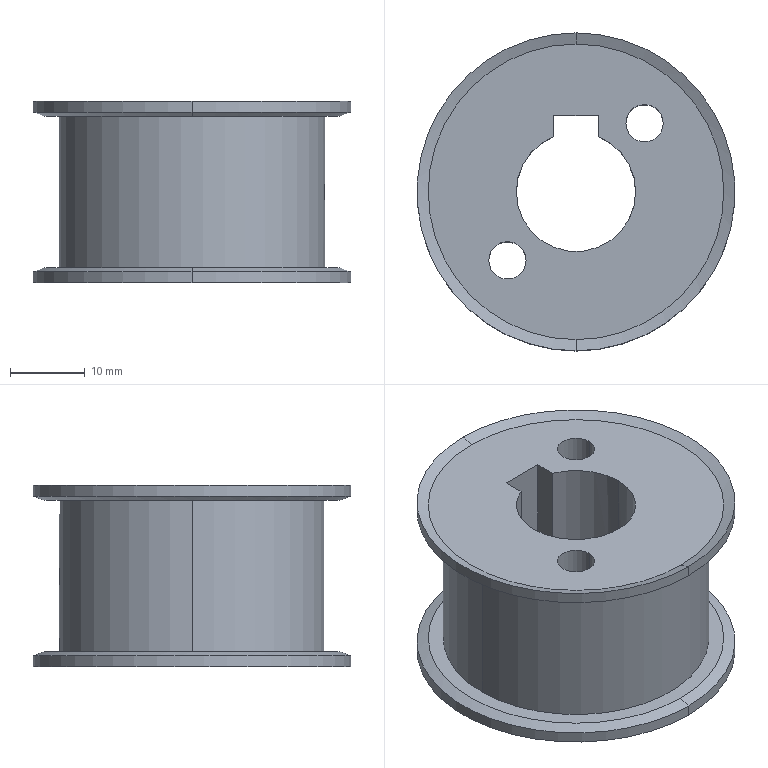Part | STEP file | Driving wheel | 1 solid | 32 faces | box 42.62 x 42.62 x 24.392 mm | volume 18419 mm3 | cylinder 17 | cone 8 | plane 7 | commonest cylinder face diameters 3.3 x4 5 x4 42.62 x4 16 x3 35.62 x2
STEP:
#1=CARTESIAN_POINT('',(-11.692,-9.192,23.3));
#2=VERTEX_POINT('',#1);
#3=CARTESIAN_POINT('',(-6.692,-9.192,23.3));
#4=VERTEX_POINT('',#3);
#5=CARTESIAN_POINT('',(-9.192,-9.192,23.3));
#6=DIRECTION('',(0.,0.,1.));
#7=DIRECTION('',(1.,0.,0.));
#8=AXIS2_PLACEMENT_3D('',#5,#6,#7);
#9=CIRCLE('',#8,2.5);
#10=EDGE_CURVE('',#2,#4,#9,.T.);
#11=ORIENTED_EDGE('',*,*,#10,.T.);
#12=CARTESIAN_POINT('',(-6.692,-9.192,0.));
#13=VERTEX_POINT('',#12);
#14=CARTESIAN_POINT('',(-6.692,-9.192,0.));
#15=DIRECTION('',(0.,0.,-1.));
#16=VECTOR('',#15,1000.);
#17=LINE('',#14,#16);
#18=EDGE_CURVE('',#4,#13,#17,.T.);
#19=ORIENTED_EDGE('',*,*,#18,.T.);
#20=CARTESIAN_POINT('',(-11.692,-9.192,0.));
#21=VERTEX_POINT('',#20);
#22=CARTESIAN_POINT('',(-9.192,-9.192,0.));
#23=DIRECTION('',(0.,0.,-1.));
#24=DIRECTION('',(-1.,0.,0.));
#25=AXIS2_PLACEMENT_3D('',#22,#23,#24);
#26=CIRCLE('',#25,2.5);
#27=EDGE_CURVE('',#13,#21,#26,.T.);
#28=ORIENTED_EDGE('',*,*,#27,.T.);
#29=CARTESIAN_POINT('',(-11.692,-9.192,0.));
#30=DIRECTION('',(0.,0.,-1.));
#31=VECTOR('',#30,1000.);
#32=LINE('',#29,#31);
#33=EDGE_CURVE('',#2,#21,#32,.T.);
#34=ORIENTED_EDGE('',*,*,#33,.F.);
#35=EDGE_LOOP('',(#11,#19,#28,#34));
#36=FACE_OUTER_BOUND('',#35,.T.);
#37=CARTESIAN_POINT('',(-9.192,-9.192,0.));
#38=DIRECTION('',(0.,0.,-1.));
#39=DIRECTION('',(-1.,0.,0.));
#40=AXIS2_PLACEMENT_3D('',#37,#38,#39);
#41=CYLINDRICAL_SURFACE('',#40,2.5);
#42=ADVANCED_FACE('',(#36),#41,.F.);
#43=CARTESIAN_POINT('',(6.692,9.192,23.3));
#44=VERTEX_POINT('',#43);
#45=CARTESIAN_POINT('',(11.692,9.192,23.3));
#46=VERTEX_POINT('',#45);
#47=CARTESIAN_POINT('',(9.192,9.192,23.3));
#48=DIRECTION('',(0.,0.,1.));
#49=DIRECTION('',(1.,0.,0.));
#50=AXIS2_PLACEMENT_3D('',#47,#48,#49);
#51=CIRCLE('',#50,2.5);
#52=EDGE_CURVE('',#44,#46,#51,.T.);
#53=ORIENTED_EDGE('',*,*,#52,.T.);
#54=CARTESIAN_POINT('',(11.692,9.192,0.));
#55=VERTEX_POINT('',#54);
#56=CARTESIAN_POINT('',(11.692,9.192,0.));
#57=DIRECTION('',(0.,0.,-1.));
#58=VECTOR('',#57,1000.);
#59=LINE('',#56,#58);
#60=EDGE_CURVE('',#46,#55,#59,.T.);
#61=ORIENTED_EDGE('',*,*,#60,.T.);
#62=CARTESIAN_POINT('',(6.692,9.192,0.));
#63=VERTEX_POINT('',#62);
#64=CARTESIAN_POINT('',(9.192,9.192,0.));
#65=DIRECTION('',(0.,0.,-1.));
#66=DIRECTION('',(-1.,0.,0.));
#67=AXIS2_PLACEMENT_3D('',#64,#65,#66);
#68=CIRCLE('',#67,2.5);
#69=EDGE_CURVE('',#55,#63,#68,.T.);
#70=ORIENTED_EDGE('',*,*,#69,.T.);
#71=CARTESIAN_POINT('',(6.692,9.192,0.));
#72=DIRECTION('',(0.,0.,-1.));
#73=VECTOR('',#72,1000.);
#74=LINE('',#71,#73);
#75=EDGE_CURVE('',#44,#63,#74,.T.);
#76=ORIENTED_EDGE('',*,*,#75,.F.);
#77=EDGE_LOOP('',(#53,#61,#70,#76));
#78=FACE_OUTER_BOUND('',#77,.T.);
#79=CARTESIAN_POINT('',(9.192,9.192,0.));
#80=DIRECTION('',(0.,0.,-1.));
#81=DIRECTION('',(-1.,0.,0.));
#82=AXIS2_PLACEMENT_3D('',#79,#80,#81);
#83=CYLINDRICAL_SURFACE('',#82,2.5);
#84=ADVANCED_FACE('',(#78),#83,.F.);
#85=CARTESIAN_POINT('',(0.,10.25,13.3));
#86=VERTEX_POINT('',#85);
#87=CARTESIAN_POINT('',(0.,10.25,10.));
#88=VERTEX_POINT('',#87);
#89=CARTESIAN_POINT('',(0.,10.25,11.65));
#90=DIRECTION('',(0.,1.,0.));
#91=DIRECTION('',(0.,0.,1.));
#92=AXIS2_PLACEMENT_3D('',#89,#90,#91);
#93=CIRCLE('',#92,1.65);
#94=EDGE_CURVE('',#86,#88,#93,.T.);
#95=ORIENTED_EDGE('',*,*,#94,.F.);
#96=CARTESIAN_POINT('',(0.,17.81,13.3));
#97=VERTEX_POINT('',#96);
#98=CARTESIAN_POINT('',(0.,17.81,13.3));
#99=DIRECTION('',(0.,1.,0.));
#100=VECTOR('',#99,1000.);
#101=LINE('',#98,#100);
#102=EDGE_CURVE('',#86,#97,#101,.T.);
#103=ORIENTED_EDGE('',*,*,#102,.T.);
#104=CARTESIAN_POINT('',(0.,17.81,10.));
#105=VERTEX_POINT('',#104);
#106=CARTESIAN_POINT('',(0.,17.81,10.));
#107=CARTESIAN_POINT('',(0.1091,17.81,10.));
#108=CARTESIAN_POINT('',(0.2163,17.809,10.011));
#109=CARTESIAN_POINT('',(0.4273,17.805,10.053));
#110=CARTESIAN_POINT('',(0.5321,17.802,10.084));
#111=CARTESIAN_POINT('',(0.7319,17.795,10.167));
#112=CARTESIAN_POINT('',(0.8267,17.791,10.218));
#113=CARTESIAN_POINT('',(1.006,17.782,10.338));
#114=CARTESIAN_POINT('',(1.091,17.777,10.407));
#115=CARTESIAN_POINT('',(1.319,17.762,10.636));
#116=CARTESIAN_POINT('',(1.442,17.752,10.82));
#117=CARTESIAN_POINT('',(1.607,17.738,11.217));
#118=CARTESIAN_POINT('',(1.65,17.733,11.434));
#119=CARTESIAN_POINT('',(1.65,17.733,11.757));
#120=CARTESIAN_POINT('',(1.639,17.734,11.866));
#121=CARTESIAN_POINT('',(1.597,17.738,12.078));
#122=CARTESIAN_POINT('',(1.566,17.741,12.181));
#123=CARTESIAN_POINT('',(1.483,17.748,12.381));
#124=CARTESIAN_POINT('',(1.432,17.752,12.477));
#125=CARTESIAN_POINT('',(1.312,17.762,12.656));
#126=CARTESIAN_POINT('',(1.244,17.767,12.739));
#127=CARTESIAN_POINT('',(1.09,17.777,12.894));
#128=CARTESIAN_POINT('',(1.007,17.782,12.962));
#129=CARTESIAN_POINT('',(0.8279,17.791,13.081));
#130=CARTESIAN_POINT('',(0.7314,17.795,13.133));
#131=CARTESIAN_POINT('',(0.5315,17.802,13.216));
#132=CARTESIAN_POINT('',(0.4287,17.805,13.247));
#133=CARTESIAN_POINT('',(0.2171,17.809,13.289));
#134=CARTESIAN_POINT('',(0.1077,17.81,13.3));
#135=CARTESIAN_POINT('',(0.,17.81,13.3));
#136=B_SPLINE_CURVE_WITH_KNOTS('',3,(#106,#107,#108,#109,#110,#111,#112,#113,#114,#115,#116,#117,#118,#119,#120,#121,#122,#123,#124,#125,#126,#127,#128,#129,#130,#131,#132,#133,#134,#135),.UNSPECIFIED.,.F.,.F.,(4,2,2,2,2,2,2,2,2,2,2,2,2,2,4),(0.,0.0003226,0.0006452,0.0009678,0.00129,0.001936,0.002581,0.002903,0.003226,0.003548,0.003871,0.004194,0.004516,0.004839,0.005161),.UNSPECIFIED.);
#137=EDGE_CURVE('',#105,#97,#136,.T.);
#138=ORIENTED_EDGE('',*,*,#137,.F.);
#139=CARTESIAN_POINT('',(0.,17.81,10.));
#140=DIRECTION('',(0.,1.,0.));
#141=VECTOR('',#140,1000.);
#142=LINE('',#139,#141);
#143=EDGE_CURVE('',#88,#105,#142,.T.);
#144=ORIENTED_EDGE('',*,*,#143,.F.);
#145=EDGE_LOOP('',(#95,#103,#138,#144));
#146=FACE_OUTER_BOUND('',#145,.T.);
#147=CARTESIAN_POINT('',(0.,17.81,11.65));
#148=DIRECTION('',(0.,1.,0.));
#149=DIRECTION('',(0.,0.,-1.));
#150=AXIS2_PLACEMENT_3D('',#147,#148,#149);
#151=CYLINDRICAL_SURFACE('',#150,1.65);
#152=ADVANCED_FACE('',(#146),#151,.F.);
#153=CARTESIAN_POINT('',(8.,0.,13.3));
#154=VERTEX_POINT('',#153);
#155=CARTESIAN_POINT('',(8.,0.,10.));
#156=VERTEX_POINT('',#155);
#157=CARTESIAN_POINT('',(8.,0.,13.3));
#158=CARTESIAN_POINT('',(8.,-0.2156,13.3));
#159=CARTESIAN_POINT('',(7.991,-0.4333,13.257));
#160=CARTESIAN_POINT('',(7.967,-0.7313,13.133));
#161=CARTESIAN_POINT('',(7.958,-0.8276,13.082));
#162=CARTESIAN_POINT('',(7.937,-1.007,12.961));
#163=CARTESIAN_POINT('',(7.926,-1.09,12.893));
#164=CARTESIAN_POINT('',(7.903,-1.242,12.741));
#165=CARTESIAN_POINT('',(7.892,-1.312,12.657));
#166=CARTESIAN_POINT('',(7.871,-1.431,12.478));
#167=CARTESIAN_POINT('',(7.862,-1.482,12.384));
#168=CARTESIAN_POINT('',(7.837,-1.607,12.083));
#169=CARTESIAN_POINT('',(7.828,-1.65,11.869));
#170=CARTESIAN_POINT('',(7.828,-1.65,11.542));
#171=CARTESIAN_POINT('',(7.83,-1.639,11.435));
#172=CARTESIAN_POINT('',(7.839,-1.597,11.223));
#173=CARTESIAN_POINT('',(7.845,-1.566,11.118));
#174=CARTESIAN_POINT('',(7.861,-1.483,10.919));
#175=CARTESIAN_POINT('',(7.871,-1.432,10.824));
#176=CARTESIAN_POINT('',(7.892,-1.312,10.644));
#177=CARTESIAN_POINT('',(7.903,-1.243,10.56));
#178=CARTESIAN_POINT('',(7.937,-1.016,10.332));
#179=CARTESIAN_POINT('',(7.959,-0.8325,10.209));
#180=CARTESIAN_POINT('',(7.983,-0.5348,10.085));
#181=CARTESIAN_POINT('',(7.989,-0.4301,10.053));
#182=CARTESIAN_POINT('',(7.998,-0.2172,10.011));
#183=CARTESIAN_POINT('',(8.,-0.1093,10.));
#184=CARTESIAN_POINT('',(8.,0.,10.));
#185=B_SPLINE_CURVE_WITH_KNOTS('',3,(#157,#158,#159,#160,#161,#162,#163,#164,#165,#166,#167,#168,#169,#170,#171,#172,#173,#174,#175,#176,#177,#178,#179,#180,#181,#182,#183,#184),.UNSPECIFIED.,.F.,.F.,(4,2,2,2,2,2,2,2,2,2,2,2,2,4),(0.005173,0.005819,0.006142,0.006465,0.006789,0.007112,0.007758,0.008081,0.008405,0.008728,0.009051,0.009697,0.01002,0.01034),.UNSPECIFIED.);
#186=EDGE_CURVE('',#154,#156,#185,.T.);
#187=ORIENTED_EDGE('',*,*,#186,.F.);
#188=CARTESIAN_POINT('',(17.81,0.,13.3));
#189=VERTEX_POINT('',#188);
#190=CARTESIAN_POINT('',(17.81,0.,13.3));
#191=DIRECTION('',(1.,0.,0.));
#192=VECTOR('',#191,1000.);
#193=LINE('',#190,#192);
#194=EDGE_CURVE('',#154,#189,#193,.T.);
#195=ORIENTED_EDGE('',*,*,#194,.T.);
#196=CARTESIAN_POINT('',(17.81,0.,10.));
#197=VERTEX_POINT('',#196);
#198=CARTESIAN_POINT('',(17.81,0.,10.));
#199=CARTESIAN_POINT('',(17.81,-0.1091,10.));
#200=CARTESIAN_POINT('',(17.809,-0.2163,10.011));
#201=CARTESIAN_POINT('',(17.805,-0.4273,10.053));
#202=CARTESIAN_POINT('',(17.802,-0.5321,10.084));
#203=CARTESIAN_POINT('',(17.795,-0.7319,10.167));
#204=CARTESIAN_POINT('',(17.791,-0.8267,10.218));
#205=CARTESIAN_POINT('',(17.782,-1.006,10.338));
#206=CARTESIAN_POINT('',(17.777,-1.091,10.407));
#207=CARTESIAN_POINT('',(17.762,-1.319,10.636));
#208=CARTESIAN_POINT('',(17.752,-1.442,10.82));
#209=CARTESIAN_POINT('',(17.738,-1.607,11.217));
#210=CARTESIAN_POINT('',(17.733,-1.65,11.434));
#211=CARTESIAN_POINT('',(17.733,-1.65,11.757));
#212=CARTESIAN_POINT('',(17.734,-1.639,11.866));
#213=CARTESIAN_POINT('',(17.738,-1.597,12.078));
#214=CARTESIAN_POINT('',(17.741,-1.566,12.181));
#215=CARTESIAN_POINT('',(17.748,-1.483,12.381));
#216=CARTESIAN_POINT('',(17.752,-1.432,12.477));
#217=CARTESIAN_POINT('',(17.762,-1.312,12.656));
#218=CARTESIAN_POINT('',(17.767,-1.244,12.739));
#219=CARTESIAN_POINT('',(17.777,-1.09,12.894));
#220=CARTESIAN_POINT('',(17.782,-1.007,12.962));
#221=CARTESIAN_POINT('',(17.791,-0.8279,13.081));
#222=CARTESIAN_POINT('',(17.795,-0.7314,13.133));
#223=CARTESIAN_POINT('',(17.802,-0.5315,13.216));
#224=CARTESIAN_POINT('',(17.805,-0.4287,13.247));
#225=CARTESIAN_POINT('',(17.809,-0.2171,13.289));
#226=CARTESIAN_POINT('',(17.81,-0.1077,13.3));
#227=CARTESIAN_POINT('',(17.81,0.,13.3));
#228=B_SPLINE_CURVE_WITH_KNOTS('',3,(#198,#199,#200,#201,#202,#203,#204,#205,#206,#207,#208,#209,#210,#211,#212,#213,#214,#215,#216,#217,#218,#219,#220,#221,#222,#223,#224,#225,#226,#227),.UNSPECIFIED.,.F.,.F.,(4,2,2,2,2,2,2,2,2,2,2,2,2,2,4),(0.,0.0003226,0.0006452,0.0009678,0.00129,0.001936,0.002581,0.002903,0.003226,0.003548,0.003871,0.004194,0.004516,0.004839,0.005161),.UNSPECIFIED.);
#229=EDGE_CURVE('',#197,#189,#228,.T.);
#230=ORIENTED_EDGE('',*,*,#229,.F.);
#231=CARTESIAN_POINT('',(17.81,0.,10.));
#232=DIRECTION('',(1.,0.,0.));
#233=VECTOR('',#232,1000.);
#234=LINE('',#231,#233);
#235=EDGE_CURVE('',#156,#197,#234,.T.);
#236=ORIENTED_EDGE('',*,*,#235,.F.);
#237=EDGE_LOOP('',(#187,#195,#230,#236));
#238=FACE_OUTER_BOUND('',#237,.T.);
#239=CARTESIAN_POINT('',(17.81,0.,11.65));
#240=DIRECTION('',(1.,0.,0.));
#241=DIRECTION('',(0.,0.,-1.));
#242=AXIS2_PLACEMENT_3D('',#239,#240,#241);
#243=CYLINDRICAL_SURFACE('',#242,1.65);
#244=ADVANCED_FACE('',(#238),#243,.F.);
#245=CARTESIAN_POINT('',(-8.,0.,0.));
#246=VERTEX_POINT('',#245);
#247=CARTESIAN_POINT('',(8.,0.,0.));
#248=VERTEX_POINT('',#247);
#249=CARTESIAN_POINT('',(0.,0.,0.));
#250=DIRECTION('',(0.,0.,1.));
#251=DIRECTION('',(1.,0.,0.));
#252=AXIS2_PLACEMENT_3D('',#249,#250,#251);
#253=CIRCLE('',#252,8.);
#254=EDGE_CURVE('',#246,#248,#253,.T.);
#255=ORIENTED_EDGE('',*,*,#254,.F.);
#256=CARTESIAN_POINT('',(-8.,0.,23.3));
#257=VERTEX_POINT('',#256);
#258=CARTESIAN_POINT('',(-8.,0.,-0.546));
#259=DIRECTION('',(0.,0.,1.));
#260=VECTOR('',#259,1000.);
#261=LINE('',#258,#260);
#262=EDGE_CURVE('',#246,#257,#261,.T.);
#263=ORIENTED_EDGE('',*,*,#262,.T.);
#264=CARTESIAN_POINT('',(8.,0.,23.3));
#265=VERTEX_POINT('',#264);
#266=CARTESIAN_POINT('',(0.,0.,23.3));
#267=DIRECTION('',(0.,0.,1.));
#268=DIRECTION('',(1.,0.,0.));
#269=AXIS2_PLACEMENT_3D('',#266,#267,#268);
#270=CIRCLE('',#269,8.);
#271=EDGE_CURVE('',#257,#265,#270,.T.);
#272=ORIENTED_EDGE('',*,*,#271,.T.);
#273=CARTESIAN_POINT('',(8.,0.,-0.546));
#274=DIRECTION('',(0.,0.,1.));
#275=VECTOR('',#274,1000.);
#276=LINE('',#273,#275);
#277=EDGE_CURVE('',#154,#265,#276,.T.);
#278=ORIENTED_EDGE('',*,*,#277,.F.);
#279=ORIENTED_EDGE('',*,*,#186,.T.);
#280=CARTESIAN_POINT('',(8.,0.,-0.546));
#281=DIRECTION('',(0.,0.,1.));
#282=VECTOR('',#281,1000.);
#283=LINE('',#280,#282);
#284=EDGE_CURVE('',#248,#156,#283,.T.);
#285=ORIENTED_EDGE('',*,*,#284,.F.);
#286=EDGE_LOOP('',(#255,#263,#272,#278,#279,#285));
#287=FACE_OUTER_BOUND('',#286,.T.);
#288=CARTESIAN_POINT('',(0.,0.,-0.546));
#289=DIRECTION('',(0.,0.,1.));
#290=DIRECTION('',(1.,0.,0.));
#291=AXIS2_PLACEMENT_3D('',#288,#289,#290);
#292=CYLINDRICAL_SURFACE('',#291,8.);
#293=ADVANCED_FACE('',(#287),#292,.F.);
#294=CARTESIAN_POINT('',(3.,7.416,0.));
#295=VERTEX_POINT('',#294);
#296=CARTESIAN_POINT('',(0.,0.,0.));
#297=DIRECTION('',(0.,0.,1.));
#298=DIRECTION('',(1.,0.,0.));
#299=AXIS2_PLACEMENT_3D('',#296,#297,#298);
#300=CIRCLE('',#299,8.);
#301=EDGE_CURVE('',#248,#295,#300,.T.);
#302=ORIENTED_EDGE('',*,*,#301,.F.);
#303=ORIENTED_EDGE('',*,*,#284,.T.);
#304=CARTESIAN_POINT('',(8.,0.,10.));
#305=CARTESIAN_POINT('',(8.,0.1093,10.));
#306=CARTESIAN_POINT('',(7.998,0.2168,10.011));
#307=CARTESIAN_POINT('',(7.989,0.4281,10.053));
#308=CARTESIAN_POINT('',(7.983,0.5331,10.085));
#309=CARTESIAN_POINT('',(7.967,0.7328,10.168));
#310=CARTESIAN_POINT('',(7.958,0.8274,10.218));
#311=CARTESIAN_POINT('',(7.937,1.007,10.338));
#312=CARTESIAN_POINT('',(7.926,1.091,10.408));
#313=CARTESIAN_POINT('',(7.892,1.319,10.635));
#314=CARTESIAN_POINT('',(7.869,1.442,10.819));
#315=CARTESIAN_POINT('',(7.838,1.606,11.216));
#316=CARTESIAN_POINT('',(7.828,1.65,11.433));
#317=CARTESIAN_POINT('',(7.828,1.65,11.757));
#318=CARTESIAN_POINT('',(7.83,1.639,11.867));
#319=CARTESIAN_POINT('',(7.839,1.597,12.079));
#320=CARTESIAN_POINT('',(7.845,1.566,12.182));
#321=CARTESIAN_POINT('',(7.87,1.441,12.482));
#322=CARTESIAN_POINT('',(7.892,1.32,12.664));
#323=CARTESIAN_POINT('',(7.926,1.09,12.893));
#324=CARTESIAN_POINT('',(7.937,1.007,12.962));
#325=CARTESIAN_POINT('',(7.957,0.8285,13.081));
#326=CARTESIAN_POINT('',(7.967,0.7318,13.133));
#327=CARTESIAN_POINT('',(7.983,0.5324,13.215));
#328=CARTESIAN_POINT('',(7.989,0.4295,13.247));
#329=CARTESIAN_POINT('',(7.998,0.2174,13.289));
#330=CARTESIAN_POINT('',(8.,0.1078,13.3));
#331=CARTESIAN_POINT('',(8.,0.,13.3));
#332=B_SPLINE_CURVE_WITH_KNOTS('',3,(#304,#305,#306,#307,#308,#309,#310,#311,#312,#313,#314,#315,#316,#317,#318,#319,#320,#321,#322,#323,#324,#325,#326,#327,#328,#329,#330,#331),.UNSPECIFIED.,.F.,.F.,(4,2,2,2,2,2,2,2,2,2,2,2,2,4),(0.,0.0003233,0.0006466,0.0009699,0.001293,0.00194,0.002586,0.00291,0.003233,0.003879,0.004203,0.004526,0.004849,0.005173),.UNSPECIFIED.);
#333=EDGE_CURVE('',#156,#154,#332,.T.);
#334=ORIENTED_EDGE('',*,*,#333,.T.);
#335=ORIENTED_EDGE('',*,*,#277,.T.);
#336=CARTESIAN_POINT('',(3.,7.416,23.3));
#337=VERTEX_POINT('',#336);
#338=CARTESIAN_POINT('',(0.,0.,23.3));
#339=DIRECTION('',(0.,0.,1.));
#340=DIRECTION('',(1.,0.,0.));
#341=AXIS2_PLACEMENT_3D('',#338,#339,#340);
#342=CIRCLE('',#341,8.);
#343=EDGE_CURVE('',#265,#337,#342,.T.);
#344=ORIENTED_EDGE('',*,*,#343,.T.);
#345=CARTESIAN_POINT('',(3.,7.416,-0.546));
#346=DIRECTION('',(0.,0.,-1.));
#347=VECTOR('',#346,1000.);
#348=LINE('',#345,#347);
#349=EDGE_CURVE('',#337,#295,#348,.T.);
#350=ORIENTED_EDGE('',*,*,#349,.T.);
#351=EDGE_LOOP('',(#302,#303,#334,#335,#344,#350));
#352=FACE_OUTER_BOUND('',#351,.T.);
#353=CARTESIAN_POINT('',(0.,0.,-0.546));
#354=DIRECTION('',(0.,0.,1.));
#355=DIRECTION('',(1.,0.,0.));
#356=AXIS2_PLACEMENT_3D('',#353,#354,#355);
#357=CYLINDRICAL_SURFACE('',#356,8.);
#358=ADVANCED_FACE('',(#352),#357,.F.);
#359=CARTESIAN_POINT('',(0.,-19.81,1.5));
#360=VERTEX_POINT('',#359);
#361=CARTESIAN_POINT('',(0.,19.81,1.5));
#362=VERTEX_POINT('',#361);
#363=CARTESIAN_POINT('',(0.,0.,1.5));
#364=DIRECTION('',(0.,0.,1.));
#365=DIRECTION('',(0.,-1.,0.));
#366=AXIS2_PLACEMENT_3D('',#363,#364,#365);
#367=CIRCLE('',#366,19.81);
#368=EDGE_CURVE('',#360,#362,#367,.T.);
#369=ORIENTED_EDGE('',*,*,#368,.F.);
#370=CARTESIAN_POINT('',(0.,-21.31,0.954));
#371=VERTEX_POINT('',#370);
#372=CARTESIAN_POINT('',(0.,-21.31,0.954));
#373=DIRECTION('',(0.,-0.9397,-0.342));
#374=VECTOR('',#373,1000.);
#375=LINE('',#372,#374);
#376=EDGE_CURVE('',#360,#371,#375,.T.);
#377=ORIENTED_EDGE('',*,*,#376,.T.);
#378=CARTESIAN_POINT('',(0.,21.31,0.954));
#379=VERTEX_POINT('',#378);
#380=CARTESIAN_POINT('',(0.,0.,0.954));
#381=DIRECTION('',(0.,0.,1.));
#382=DIRECTION('',(0.,-1.,0.));
#383=AXIS2_PLACEMENT_3D('',#380,#381,#382);
#384=CIRCLE('',#383,21.31);
#385=EDGE_CURVE('',#371,#379,#384,.T.);
#386=ORIENTED_EDGE('',*,*,#385,.T.);
#387=CARTESIAN_POINT('',(0.,21.31,0.954));
#388=DIRECTION('',(0.,0.9397,-0.342));
#389=VECTOR('',#388,1000.);
#390=LINE('',#387,#389);
#391=EDGE_CURVE('',#362,#379,#390,.T.);
#392=ORIENTED_EDGE('',*,*,#391,.F.);
#393=EDGE_LOOP('',(#369,#377,#386,#392));
#394=FACE_OUTER_BOUND('',#393,.T.);
#395=CARTESIAN_POINT('',(0.,0.,0.954));
#396=DIRECTION('',(0.,0.,-1.));
#397=DIRECTION('',(0.,1.,0.));
#398=AXIS2_PLACEMENT_3D('',#395,#396,#397);
#399=CONICAL_SURFACE('',#398,21.31,1.222);
#400=ADVANCED_FACE('',(#394),#399,.T.);
#401=CARTESIAN_POINT('',(0.,-21.31,-0.546));
#402=VERTEX_POINT('',#401);
#403=CARTESIAN_POINT('',(0.,21.31,-0.546));
#404=VERTEX_POINT('',#403);
#405=CARTESIAN_POINT('',(0.,0.,-0.546));
#406=DIRECTION('',(0.,0.,1.));
#407=DIRECTION('',(0.,-1.,0.));
#408=AXIS2_PLACEMENT_3D('',#405,#406,#407);
#409=CIRCLE('',#408,21.31);
#410=EDGE_CURVE('',#402,#404,#409,.T.);
#411=ORIENTED_EDGE('',*,*,#410,.T.);
#412=CARTESIAN_POINT('',(0.,21.31,23.3));
#413=DIRECTION('',(0.,0.,1.));
#414=VECTOR('',#413,1000.);
#415=LINE('',#412,#414);
#416=EDGE_CURVE('',#404,#379,#415,.T.);
#417=ORIENTED_EDGE('',*,*,#416,.T.);
#418=ORIENTED_EDGE('',*,*,#385,.F.);
#419=CARTESIAN_POINT('',(0.,-21.31,23.3));
#420=DIRECTION('',(0.,0.,1.));
#421=VECTOR('',#420,1000.);
#422=LINE('',#419,#421);
#423=EDGE_CURVE('',#402,#371,#422,.T.);
#424=ORIENTED_EDGE('',*,*,#423,.F.);
#425=EDGE_LOOP('',(#411,#417,#418,#424));
#426=FACE_OUTER_BOUND('',#425,.T.);
#427=CARTESIAN_POINT('',(0.,0.,23.3));
#428=DIRECTION('',(0.,0.,1.));
#429=DIRECTION('',(0.,-1.,0.));
#430=AXIS2_PLACEMENT_3D('',#427,#428,#429);
#431=CYLINDRICAL_SURFACE('',#430,21.31);
#432=ADVANCED_FACE('',(#426),#431,.T.);
#433=CARTESIAN_POINT('',(0.,19.81,0.));
#434=VERTEX_POINT('',#433);
#435=CARTESIAN_POINT('',(0.,-19.81,0.));
#436=VERTEX_POINT('',#435);
#437=CARTESIAN_POINT('',(0.,0.,0.));
#438=DIRECTION('',(0.,0.,1.));
#439=DIRECTION('',(0.,-1.,0.));
#440=AXIS2_PLACEMENT_3D('',#437,#438,#439);
#441=CIRCLE('',#440,19.81);
#442=EDGE_CURVE('',#434,#436,#441,.T.);
#443=ORIENTED_EDGE('',*,*,#442,.T.);
#444=CARTESIAN_POINT('',(0.,-19.81,0.));
#445=DIRECTION('',(0.,-0.9397,-0.342));
#446=VECTOR('',#445,1000.);
#447=LINE('',#444,#446);
#448=EDGE_CURVE('',#436,#402,#447,.T.);
#449=ORIENTED_EDGE('',*,*,#448,.T.);
#450=CARTESIAN_POINT('',(0.,0.,-0.546));
#451=DIRECTION('',(0.,0.,1.));
#452=DIRECTION('',(0.,-1.,0.));
#453=AXIS2_PLACEMENT_3D('',#450,#451,#452);
#454=CIRCLE('',#453,21.31);
#455=EDGE_CURVE('',#404,#402,#454,.T.);
#456=ORIENTED_EDGE('',*,*,#455,.F.);
#457=CARTESIAN_POINT('',(0.,19.81,0.));
#458=DIRECTION('',(0.,0.9397,-0.342));
#459=VECTOR('',#458,1000.);
#460=LINE('',#457,#459);
#461=EDGE_CURVE('',#434,#404,#460,.T.);
#462=ORIENTED_EDGE('',*,*,#461,.F.);
#463=EDGE_LOOP('',(#443,#449,#456,#462));
#464=FACE_OUTER_BOUND('',#463,.T.);
#465=CARTESIAN_POINT('',(0.,0.,0.));
#466=DIRECTION('',(0.,0.,-1.));
#467=DIRECTION('',(0.,1.,0.));
#468=AXIS2_PLACEMENT_3D('',#465,#466,#467);
#469=CONICAL_SURFACE('',#468,19.81,1.222);
#470=ADVANCED_FACE('',(#464),#469,.F.);
#471=CARTESIAN_POINT('',(0.,19.81,23.3));
#472=VERTEX_POINT('',#471);
#473=CARTESIAN_POINT('',(0.,-19.81,23.3));
#474=VERTEX_POINT('',#473);
#475=CARTESIAN_POINT('',(0.,0.,23.3));
#476=DIRECTION('',(0.,0.,1.));
#477=DIRECTION('',(0.,-1.,0.));
#478=AXIS2_PLACEMENT_3D('',#475,#476,#477);
#479=CIRCLE('',#478,19.81);
#480=EDGE_CURVE('',#472,#474,#479,.T.);
#481=ORIENTED_EDGE('',*,*,#480,.F.);
#482=CARTESIAN_POINT('',(0.,21.31,23.846));
#483=VERTEX_POINT('',#482);
#484=CARTESIAN_POINT('',(0.,21.31,23.846));
#485=DIRECTION('',(0.,0.9397,0.342));
#486=VECTOR('',#485,1000.);
#487=LINE('',#484,#486);
#488=EDGE_CURVE('',#472,#483,#487,.T.);
#489=ORIENTED_EDGE('',*,*,#488,.T.);
#490=CARTESIAN_POINT('',(0.,-21.31,23.846));
#491=VERTEX_POINT('',#490);
#492=CARTESIAN_POINT('',(0.,0.,23.846));
#493=DIRECTION('',(0.,0.,1.));
#494=DIRECTION('',(0.,-1.,0.));
#495=AXIS2_PLACEMENT_3D('',#492,#493,#494);
#496=CIRCLE('',#495,21.31);
#497=EDGE_CURVE('',#483,#491,#496,.T.);
#498=ORIENTED_EDGE('',*,*,#497,.T.);
#499=CARTESIAN_POINT('',(0.,-21.31,23.846));
#500=DIRECTION('',(0.,-0.9397,0.342));
#501=VECTOR('',#500,1000.);
#502=LINE('',#499,#501);
#503=EDGE_CURVE('',#474,#491,#502,.T.);
#504=ORIENTED_EDGE('',*,*,#503,.F.);
#505=EDGE_LOOP('',(#481,#489,#498,#504));
#506=FACE_OUTER_BOUND('',#505,.T.);
#507=CARTESIAN_POINT('',(0.,0.,23.846));
#508=DIRECTION('',(0.,0.,1.));
#509=DIRECTION('',(0.,-1.,0.));
#510=AXIS2_PLACEMENT_3D('',#507,#508,#509);
#511=CONICAL_SURFACE('',#510,21.31,1.222);
#512=ADVANCED_FACE('',(#506),#511,.F.);
#513=CARTESIAN_POINT('',(0.,-21.31,22.346));
#514=VERTEX_POINT('',#513);
#515=CARTESIAN_POINT('',(0.,21.31,22.346));
#516=VERTEX_POINT('',#515);
#517=CARTESIAN_POINT('',(0.,0.,22.346));
#518=DIRECTION('',(0.,0.,1.));
#519=DIRECTION('',(0.,-1.,0.));
#520=AXIS2_PLACEMENT_3D('',#517,#518,#519);
#521=CIRCLE('',#520,21.31);
#522=EDGE_CURVE('',#514,#516,#521,.T.);
#523=ORIENTED_EDGE('',*,*,#522,.T.);
#524=CARTESIAN_POINT('',(0.,21.31,23.3));
#525=DIRECTION('',(0.,0.,1.));
#526=VECTOR('',#525,1000.);
#527=LINE('',#524,#526);
#528=EDGE_CURVE('',#516,#483,#527,.T.);
#529=ORIENTED_EDGE('',*,*,#528,.T.);
#530=CARTESIAN_POINT('',(0.,0.,23.846));
#531=DIRECTION('',(0.,0.,1.));
#532=DIRECTION('',(0.,-1.,0.));
#533=AXIS2_PLACEMENT_3D('',#530,#531,#532);
#534=CIRCLE('',#533,21.31);
#535=EDGE_CURVE('',#491,#483,#534,.T.);
#536=ORIENTED_EDGE('',*,*,#535,.F.);
#537=CARTESIAN_POINT('',(0.,-21.31,23.3));
#538=DIRECTION('',(0.,0.,1.));
#539=VECTOR('',#538,1000.);
#540=LINE('',#537,#539);
#541=EDGE_CURVE('',#514,#491,#540,.T.);
#542=ORIENTED_EDGE('',*,*,#541,.F.);
#543=EDGE_LOOP('',(#523,#529,#536,#542));
#544=FACE_OUTER_BOUND('',#543,.T.);
#545=CARTESIAN_POINT('',(0.,0.,23.3));
#546=DIRECTION('',(0.,0.,1.));
#547=DIRECTION('',(0.,-1.,0.));
#548=AXIS2_PLACEMENT_3D('',#545,#546,#547);
#549=CYLINDRICAL_SURFACE('',#548,21.31);
#550=ADVANCED_FACE('',(#544),#549,.T.);
#551=CARTESIAN_POINT('',(0.,-19.81,21.8));
#552=VERTEX_POINT('',#551);
#553=CARTESIAN_POINT('',(0.,19.81,21.8));
#554=VERTEX_POINT('',#553);
#555=CARTESIAN_POINT('',(0.,0.,21.8));
#556=DIRECTION('',(0.,0.,1.));
#557=DIRECTION('',(0.,-1.,0.));
#558=AXIS2_PLACEMENT_3D('',#555,#556,#557);
#559=CIRCLE('',#558,19.81);
#560=EDGE_CURVE('',#552,#554,#559,.T.);
#561=ORIENTED_EDGE('',*,*,#560,.T.);
#562=CARTESIAN_POINT('',(0.,19.81,21.8));
#563=DIRECTION('',(0.,0.9397,0.342));
#564=VECTOR('',#563,1000.);
#565=LINE('',#562,#564);
#566=EDGE_CURVE('',#554,#516,#565,.T.);
#567=ORIENTED_EDGE('',*,*,#566,.T.);
#568=ORIENTED_EDGE('',*,*,#522,.F.);
#569=CARTESIAN_POINT('',(0.,-19.81,21.8));
#570=DIRECTION('',(0.,-0.9397,0.342));
#571=VECTOR('',#570,1000.);
#572=LINE('',#569,#571);
#573=EDGE_CURVE('',#552,#514,#572,.T.);
#574=ORIENTED_EDGE('',*,*,#573,.F.);
#575=EDGE_LOOP('',(#561,#567,#568,#574));
#576=FACE_OUTER_BOUND('',#575,.T.);
#577=CARTESIAN_POINT('',(0.,0.,21.8));
#578=DIRECTION('',(0.,0.,1.));
#579=DIRECTION('',(0.,-1.,0.));
#580=AXIS2_PLACEMENT_3D('',#577,#578,#579);
#581=CONICAL_SURFACE('',#580,19.81,1.222);
#582=ADVANCED_FACE('',(#576),#581,.T.);
#583=ORIENTED_EDGE('',*,*,#137,.T.);
#584=CARTESIAN_POINT('',(0.,17.81,13.3));
#585=CARTESIAN_POINT('',(-0.2154,17.81,13.3));
#586=CARTESIAN_POINT('',(-0.4325,17.806,13.257));
#587=CARTESIAN_POINT('',(-0.8297,17.792,13.092));
#588=CARTESIAN_POINT('',(-1.014,17.782,12.97));
#589=CARTESIAN_POINT('',(-1.242,17.767,12.742));
#590=CARTESIAN_POINT('',(-1.312,17.762,12.657));
#591=CARTESIAN_POINT('',(-1.432,17.752,12.477));
#592=CARTESIAN_POINT('',(-1.482,17.748,12.383));
#593=CARTESIAN_POINT('',(-1.565,17.741,12.183));
#594=CARTESIAN_POINT('',(-1.597,17.738,12.078));
#595=CARTESIAN_POINT('',(-1.639,17.734,11.867));
#596=CARTESIAN_POINT('',(-1.65,17.733,11.76));
#597=CARTESIAN_POINT('',(-1.65,17.733,11.542));
#598=CARTESIAN_POINT('',(-1.639,17.734,11.435));
#599=CARTESIAN_POINT('',(-1.598,17.738,11.224));
#600=CARTESIAN_POINT('',(-1.566,17.741,11.119));
#601=CARTESIAN_POINT('',(-1.483,17.748,10.919));
#602=CARTESIAN_POINT('',(-1.433,17.752,10.824));
#603=CARTESIAN_POINT('',(-1.313,17.762,10.645));
#604=CARTESIAN_POINT('',(-1.244,17.767,10.56));
#605=CARTESIAN_POINT('',(-1.015,17.782,10.332));
#606=CARTESIAN_POINT('',(-0.8317,17.792,10.209));
#607=CARTESIAN_POINT('',(-0.4348,17.806,10.044));
#608=CARTESIAN_POINT('',(-0.2181,17.81,10.));
#609=CARTESIAN_POINT('',(0.,17.81,10.));
#610=B_SPLINE_CURVE_WITH_KNOTS('',3,(#584,#585,#586,#587,#588,#589,#590,#591,#592,#593,#594,#595,#596,#597,#598,#599,#600,#601,#602,#603,#604,#605,#606,#607,#608,#609),.UNSPECIFIED.,.F.,.F.,(4,2,2,2,2,2,2,2,2,2,2,2,4),(0.005161,0.005806,0.006451,0.006774,0.007096,0.007419,0.007742,0.008064,0.008387,0.008709,0.009032,0.009677,0.01032),.UNSPECIFIED.);
#611=EDGE_CURVE('',#97,#105,#610,.T.);
#612=ORIENTED_EDGE('',*,*,#611,.T.);
#613=EDGE_LOOP('',(#583,#612));
#614=FACE_BOUND('',#613,.T.);
#615=CARTESIAN_POINT('',(17.81,0.,21.8));
#616=VERTEX_POINT('',#615);
#617=CARTESIAN_POINT('',(-17.81,0.,21.8));
#618=VERTEX_POINT('',#617);
#619=CARTESIAN_POINT('',(0.,0.,21.8));
#620=DIRECTION('',(0.,0.,1.));
#621=DIRECTION('',(0.,-1.,0.));
#622=AXIS2_PLACEMENT_3D('',#619,#620,#621);
#623=CIRCLE('',#622,17.81);
#624=EDGE_CURVE('',#616,#618,#623,.T.);
#625=ORIENTED_EDGE('',*,*,#624,.F.);
#626=CARTESIAN_POINT('',(17.81,0.,23.3));
#627=DIRECTION('',(0.,0.,-1.));
#628=VECTOR('',#627,1000.);
#629=LINE('',#626,#628);
#630=EDGE_CURVE('',#616,#189,#629,.T.);
#631=ORIENTED_EDGE('',*,*,#630,.T.);
#632=CARTESIAN_POINT('',(17.81,0.,13.3));
#633=CARTESIAN_POINT('',(17.81,0.2154,13.3));
#634=CARTESIAN_POINT('',(17.806,0.4325,13.257));
#635=CARTESIAN_POINT('',(17.792,0.8297,13.092));
#636=CARTESIAN_POINT('',(17.782,1.014,12.97));
#637=CARTESIAN_POINT('',(17.767,1.242,12.742));
#638=CARTESIAN_POINT('',(17.762,1.312,12.657));
#639=CARTESIAN_POINT('',(17.752,1.432,12.477));
#640=CARTESIAN_POINT('',(17.748,1.482,12.383));
#641=CARTESIAN_POINT('',(17.741,1.565,12.183));
#642=CARTESIAN_POINT('',(17.738,1.597,12.078));
#643=CARTESIAN_POINT('',(17.734,1.639,11.867));
#644=CARTESIAN_POINT('',(17.733,1.65,11.76));
#645=CARTESIAN_POINT('',(17.733,1.65,11.542));
#646=CARTESIAN_POINT('',(17.734,1.639,11.435));
#647=CARTESIAN_POINT('',(17.738,1.598,11.224));
#648=CARTESIAN_POINT('',(17.741,1.566,11.119));
#649=CARTESIAN_POINT('',(17.748,1.483,10.919));
#650=CARTESIAN_POINT('',(17.752,1.433,10.824));
#651=CARTESIAN_POINT('',(17.762,1.313,10.645));
#652=CARTESIAN_POINT('',(17.767,1.244,10.56));
#653=CARTESIAN_POINT('',(17.782,1.015,10.332));
#654=CARTESIAN_POINT('',(17.792,0.8317,10.209));
#655=CARTESIAN_POINT('',(17.806,0.4348,10.044));
#656=CARTESIAN_POINT('',(17.81,0.2181,10.));
#657=CARTESIAN_POINT('',(17.81,0.,10.));
#658=B_SPLINE_CURVE_WITH_KNOTS('',3,(#632,#633,#634,#635,#636,#637,#638,#639,#640,#641,#642,#643,#644,#645,#646,#647,#648,#649,#650,#651,#652,#653,#654,#655,#656,#657),.UNSPECIFIED.,.F.,.F.,(4,2,2,2,2,2,2,2,2,2,2,2,4),(0.005161,0.005806,0.006451,0.006774,0.007096,0.007419,0.007742,0.008064,0.008387,0.008709,0.009032,0.009677,0.01032),.UNSPECIFIED.);
#659=EDGE_CURVE('',#189,#197,#658,.T.);
#660=ORIENTED_EDGE('',*,*,#659,.T.);
#661=CARTESIAN_POINT('',(17.81,0.,1.5));
#662=VERTEX_POINT('',#661);
#663=CARTESIAN_POINT('',(17.81,0.,23.3));
#664=DIRECTION('',(0.,0.,-1.));
#665=VECTOR('',#664,1000.);
#666=LINE('',#663,#665);
#667=EDGE_CURVE('',#197,#662,#666,.T.);
#668=ORIENTED_EDGE('',*,*,#667,.T.);
#669=CARTESIAN_POINT('',(-17.81,0.,1.5));
#670=VERTEX_POINT('',#669);
#671=CARTESIAN_POINT('',(0.,0.,1.5));
#672=DIRECTION('',(0.,0.,-1.));
#673=DIRECTION('',(0.,1.,0.));
#674=AXIS2_PLACEMENT_3D('',#671,#672,#673);
#675=CIRCLE('',#674,17.81);
#676=EDGE_CURVE('',#670,#662,#675,.T.);
#677=ORIENTED_EDGE('',*,*,#676,.F.);
#678=CARTESIAN_POINT('',(-17.81,0.,23.3));
#679=DIRECTION('',(0.,0.,-1.));
#680=VECTOR('',#679,1000.);
#681=LINE('',#678,#680);
#682=EDGE_CURVE('',#618,#670,#681,.T.);
#683=ORIENTED_EDGE('',*,*,#682,.F.);
#684=EDGE_LOOP('',(#625,#631,#660,#668,#677,#683));
#685=FACE_OUTER_BOUND('',#684,.T.);
#686=CARTESIAN_POINT('',(0.,0.,23.3));
#687=DIRECTION('',(0.,0.,-1.));
#688=DIRECTION('',(-1.,0.,0.));
#689=AXIS2_PLACEMENT_3D('',#686,#687,#688);
#690=CYLINDRICAL_SURFACE('',#689,17.81);
#691=ADVANCED_FACE('',(#614,#685),#690,.T.);
#692=ORIENTED_EDGE('',*,*,#630,.F.);
#693=CARTESIAN_POINT('',(0.,0.,21.8));
#694=DIRECTION('',(0.,0.,1.));
#695=DIRECTION('',(0.,-1.,0.));
#696=AXIS2_PLACEMENT_3D('',#693,#694,#695);
#697=CIRCLE('',#696,17.81);
#698=EDGE_CURVE('',#618,#616,#697,.T.);
#699=ORIENTED_EDGE('',*,*,#698,.F.);
#700=ORIENTED_EDGE('',*,*,#682,.T.);
#701=CARTESIAN_POINT('',(0.,0.,1.5));
#702=DIRECTION('',(0.,0.,-1.));
#703=DIRECTION('',(0.,1.,0.));
#704=AXIS2_PLACEMENT_3D('',#701,#702,#703);
#705=CIRCLE('',#704,17.81);
#706=EDGE_CURVE('',#662,#670,#705,.T.);
#707=ORIENTED_EDGE('',*,*,#706,.F.);
#708=ORIENTED_EDGE('',*,*,#667,.F.);
#709=ORIENTED_EDGE('',*,*,#229,.T.);
#710=EDGE_LOOP('',(#692,#699,#700,#707,#708,#709));
#711=FACE_OUTER_BOUND('',#710,.T.);
#712=CARTESIAN_POINT('',(0.,0.,23.3));
#713=DIRECTION('',(0.,0.,-1.));
#714=DIRECTION('',(-1.,0.,0.));
#715=AXIS2_PLACEMENT_3D('',#712,#713,#714);
#716=CYLINDRICAL_SURFACE('',#715,17.81);
#717=ADVANCED_FACE('',(#711),#716,.T.);
#718=ORIENTED_EDGE('',*,*,#560,.F.);
#719=CARTESIAN_POINT('',(0.,0.,21.8));
#720=DIRECTION('',(0.,0.,1.));
#721=DIRECTION('',(0.,-1.,0.));
#722=AXIS2_PLACEMENT_3D('',#719,#720,#721);
#723=CIRCLE('',#722,19.81);
#724=EDGE_CURVE('',#554,#552,#723,.T.);
#725=ORIENTED_EDGE('',*,*,#724,.F.);
#726=EDGE_LOOP('',(#718,#725));
#727=FACE_OUTER_BOUND('',#726,.T.);
#728=ORIENTED_EDGE('',*,*,#698,.T.);
#729=ORIENTED_EDGE('',*,*,#624,.T.);
#730=EDGE_LOOP('',(#728,#729));
#731=FACE_BOUND('',#730,.T.);
#732=CARTESIAN_POINT('',(0.,17.81,21.8));
#733=DIRECTION('',(0.,0.,1.));
#734=DIRECTION('',(0.,-1.,0.));
#735=AXIS2_PLACEMENT_3D('',#732,#733,#734);
#736=PLANE('',#735);
#737=ADVANCED_FACE('',(#727,#731),#736,.F.);
#738=ORIENTED_EDGE('',*,*,#566,.F.);
#739=ORIENTED_EDGE('',*,*,#724,.T.);
#740=ORIENTED_EDGE('',*,*,#573,.T.);
#741=CARTESIAN_POINT('',(0.,0.,22.346));
#742=DIRECTION('',(0.,0.,1.));
#743=DIRECTION('',(0.,-1.,0.));
#744=AXIS2_PLACEMENT_3D('',#741,#742,#743);
#745=CIRCLE('',#744,21.31);
#746=EDGE_CURVE('',#516,#514,#745,.T.);
#747=ORIENTED_EDGE('',*,*,#746,.F.);
#748=EDGE_LOOP('',(#738,#739,#740,#747));
#749=FACE_OUTER_BOUND('',#748,.T.);
#750=CARTESIAN_POINT('',(0.,0.,21.8));
#751=DIRECTION('',(0.,0.,1.));
#752=DIRECTION('',(0.,-1.,0.));
#753=AXIS2_PLACEMENT_3D('',#750,#751,#752);
#754=CONICAL_SURFACE('',#753,19.81,1.222);
#755=ADVANCED_FACE('',(#749),#754,.T.);
#756=ORIENTED_EDGE('',*,*,#528,.F.);
#757=ORIENTED_EDGE('',*,*,#746,.T.);
#758=ORIENTED_EDGE('',*,*,#541,.T.);
#759=ORIENTED_EDGE('',*,*,#497,.F.);
#760=EDGE_LOOP('',(#756,#757,#758,#759));
#761=FACE_OUTER_BOUND('',#760,.T.);
#762=CARTESIAN_POINT('',(0.,0.,23.3));
#763=DIRECTION('',(0.,0.,1.));
#764=DIRECTION('',(0.,-1.,0.));
#765=AXIS2_PLACEMENT_3D('',#762,#763,#764);
#766=CYLINDRICAL_SURFACE('',#765,21.31);
#767=ADVANCED_FACE('',(#761),#766,.T.);
#768=ORIENTED_EDGE('',*,*,#488,.F.);
#769=CARTESIAN_POINT('',(0.,0.,23.3));
#770=DIRECTION('',(0.,0.,1.));
#771=DIRECTION('',(0.,-1.,0.));
#772=AXIS2_PLACEMENT_3D('',#769,#770,#771);
#773=CIRCLE('',#772,19.81);
#774=EDGE_CURVE('',#474,#472,#773,.T.);
#775=ORIENTED_EDGE('',*,*,#774,.F.);
#776=ORIENTED_EDGE('',*,*,#503,.T.);
#777=ORIENTED_EDGE('',*,*,#535,.T.);
#778=EDGE_LOOP('',(#768,#775,#776,#777));
#779=FACE_OUTER_BOUND('',#778,.T.);
#780=CARTESIAN_POINT('',(0.,0.,23.846));
#781=DIRECTION('',(0.,0.,1.));
#782=DIRECTION('',(0.,-1.,0.));
#783=AXIS2_PLACEMENT_3D('',#780,#781,#782);
#784=CONICAL_SURFACE('',#783,21.31,1.222);
#785=ADVANCED_FACE('',(#779),#784,.F.);
#786=ORIENTED_EDGE('',*,*,#10,.F.);
#787=CARTESIAN_POINT('',(-9.192,-9.192,23.3));
#788=DIRECTION('',(0.,0.,1.));
#789=DIRECTION('',(1.,0.,0.));
#790=AXIS2_PLACEMENT_3D('',#787,#788,#789);
#791=CIRCLE('',#790,2.5);
#792=EDGE_CURVE('',#4,#2,#791,.T.);
#793=ORIENTED_EDGE('',*,*,#792,.F.);
#794=EDGE_LOOP('',(#786,#793));
#795=FACE_BOUND('',#794,.T.);
#796=ORIENTED_EDGE('',*,*,#52,.F.);
#797=CARTESIAN_POINT('',(9.192,9.192,23.3));
#798=DIRECTION('',(0.,0.,1.));
#799=DIRECTION('',(1.,0.,0.));
#800=AXIS2_PLACEMENT_3D('',#797,#798,#799);
#801=CIRCLE('',#800,2.5);
#802=EDGE_CURVE('',#46,#44,#801,.T.);
#803=ORIENTED_EDGE('',*,*,#802,.F.);
#804=EDGE_LOOP('',(#796,#803));
#805=FACE_BOUND('',#804,.T.);
#806=CARTESIAN_POINT('',(3.,10.25,23.3));
#807=VERTEX_POINT('',#806);
#808=CARTESIAN_POINT('',(3.,0.,23.3));
#809=DIRECTION('',(0.,1.,0.));
#810=VECTOR('',#809,1000.);
#811=LINE('',#808,#810);
#812=EDGE_CURVE('',#337,#807,#811,.T.);
#813=ORIENTED_EDGE('',*,*,#812,.F.);
#814=ORIENTED_EDGE('',*,*,#343,.F.);
#815=ORIENTED_EDGE('',*,*,#271,.F.);
#816=CARTESIAN_POINT('',(-3.,7.416,23.3));
#817=VERTEX_POINT('',#816);
#818=CARTESIAN_POINT('',(0.,0.,23.3));
#819=DIRECTION('',(0.,0.,1.));
#820=DIRECTION('',(1.,0.,0.));
#821=AXIS2_PLACEMENT_3D('',#818,#819,#820);
#822=CIRCLE('',#821,8.);
#823=EDGE_CURVE('',#817,#257,#822,.T.);
#824=ORIENTED_EDGE('',*,*,#823,.F.);
#825=CARTESIAN_POINT('',(-3.,10.25,23.3));
#826=VERTEX_POINT('',#825);
#827=CARTESIAN_POINT('',(-3.,0.,23.3));
#828=DIRECTION('',(0.,-1.,0.));
#829=VECTOR('',#828,1000.);
#830=LINE('',#827,#829);
#831=EDGE_CURVE('',#826,#817,#830,.T.);
#832=ORIENTED_EDGE('',*,*,#831,.F.);
#833=CARTESIAN_POINT('',(0.,10.25,23.3));
#834=DIRECTION('',(-1.,0.,0.));
#835=VECTOR('',#834,1000.);
#836=LINE('',#833,#835);
#837=EDGE_CURVE('',#807,#826,#836,.T.);
#838=ORIENTED_EDGE('',*,*,#837,.F.);
#839=EDGE_LOOP('',(#813,#814,#815,#824,#832,#838));
#840=FACE_BOUND('',#839,.T.);
#841=ORIENTED_EDGE('',*,*,#774,.T.);
#842=ORIENTED_EDGE('',*,*,#480,.T.);
#843=EDGE_LOOP('',(#841,#842));
#844=FACE_OUTER_BOUND('',#843,.T.);
#845=CARTESIAN_POINT('',(0.,0.,23.3));
#846=DIRECTION('',(0.,0.,1.));
#847=DIRECTION('',(1.,0.,0.));
#848=AXIS2_PLACEMENT_3D('',#845,#846,#847);
#849=PLANE('',#848);
#850=ADVANCED_FACE('',(#795,#805,#840,#844),#849,.T.);
#851=ORIENTED_EDGE('',*,*,#676,.T.);
#852=ORIENTED_EDGE('',*,*,#706,.T.);
#853=EDGE_LOOP('',(#851,#852));
#854=FACE_BOUND('',#853,.T.);
#855=CARTESIAN_POINT('',(0.,0.,1.5));
#856=DIRECTION('',(0.,0.,1.));
#857=DIRECTION('',(0.,-1.,0.));
#858=AXIS2_PLACEMENT_3D('',#855,#856,#857);
#859=CIRCLE('',#858,19.81);
#860=EDGE_CURVE('',#362,#360,#859,.T.);
#861=ORIENTED_EDGE('',*,*,#860,.T.);
#862=ORIENTED_EDGE('',*,*,#368,.T.);
#863=EDGE_LOOP('',(#861,#862));
#864=FACE_OUTER_BOUND('',#863,.T.);
#865=CARTESIAN_POINT('',(0.,17.81,1.5));
#866=DIRECTION('',(0.,0.,-1.));
#867=DIRECTION('',(0.,1.,0.));
#868=AXIS2_PLACEMENT_3D('',#865,#866,#867);
#869=PLANE('',#868);
#870=ADVANCED_FACE('',(#854,#864),#869,.F.);
#871=ORIENTED_EDGE('',*,*,#448,.F.);
#872=CARTESIAN_POINT('',(0.,0.,0.));
#873=DIRECTION('',(0.,0.,1.));
#874=DIRECTION('',(0.,-1.,0.));
#875=AXIS2_PLACEMENT_3D('',#872,#873,#874);
#876=CIRCLE('',#875,19.81);
#877=EDGE_CURVE('',#436,#434,#876,.T.);
#878=ORIENTED_EDGE('',*,*,#877,.T.);
#879=ORIENTED_EDGE('',*,*,#461,.T.);
#880=ORIENTED_EDGE('',*,*,#410,.F.);
#881=EDGE_LOOP('',(#871,#878,#879,#880));
#882=FACE_OUTER_BOUND('',#881,.T.);
#883=CARTESIAN_POINT('',(0.,0.,0.));
#884=DIRECTION('',(0.,0.,-1.));
#885=DIRECTION('',(0.,1.,0.));
#886=AXIS2_PLACEMENT_3D('',#883,#884,#885);
#887=CONICAL_SURFACE('',#886,19.81,1.222);
#888=ADVANCED_FACE('',(#882),#887,.F.);
#889=ORIENTED_EDGE('',*,*,#416,.F.);
#890=ORIENTED_EDGE('',*,*,#455,.T.);
#891=ORIENTED_EDGE('',*,*,#423,.T.);
#892=CARTESIAN_POINT('',(0.,0.,0.954));
#893=DIRECTION('',(0.,0.,1.));
#894=DIRECTION('',(0.,-1.,0.));
#895=AXIS2_PLACEMENT_3D('',#892,#893,#894);
#896=CIRCLE('',#895,21.31);
#897=EDGE_CURVE('',#379,#371,#896,.T.);
#898=ORIENTED_EDGE('',*,*,#897,.F.);
#899=EDGE_LOOP('',(#889,#890,#891,#898));
#900=FACE_OUTER_BOUND('',#899,.T.);
#901=CARTESIAN_POINT('',(0.,0.,23.3));
#902=DIRECTION('',(0.,0.,1.));
#903=DIRECTION('',(0.,-1.,0.));
#904=AXIS2_PLACEMENT_3D('',#901,#902,#903);
#905=CYLINDRICAL_SURFACE('',#904,21.31);
#906=ADVANCED_FACE('',(#900),#905,.T.);
#907=ORIENTED_EDGE('',*,*,#376,.F.);
#908=ORIENTED_EDGE('',*,*,#860,.F.);
#909=ORIENTED_EDGE('',*,*,#391,.T.);
#910=ORIENTED_EDGE('',*,*,#897,.T.);
#911=EDGE_LOOP('',(#907,#908,#909,#910));
#912=FACE_OUTER_BOUND('',#911,.T.);
#913=CARTESIAN_POINT('',(0.,0.,0.954));
#914=DIRECTION('',(0.,0.,-1.));
#915=DIRECTION('',(0.,1.,0.));
#916=AXIS2_PLACEMENT_3D('',#913,#914,#915);
#917=CONICAL_SURFACE('',#916,21.31,1.222);
#918=ADVANCED_FACE('',(#912),#917,.T.);
#919=CARTESIAN_POINT('',(-9.192,-9.192,0.));
#920=DIRECTION('',(0.,0.,-1.));
#921=DIRECTION('',(-1.,0.,0.));
#922=AXIS2_PLACEMENT_3D('',#919,#920,#921);
#923=CIRCLE('',#922,2.5);
#924=EDGE_CURVE('',#21,#13,#923,.T.);
#925=ORIENTED_EDGE('',*,*,#924,.F.);
#926=ORIENTED_EDGE('',*,*,#27,.F.);
#927=EDGE_LOOP('',(#925,#926));
#928=FACE_BOUND('',#927,.T.);
#929=CARTESIAN_POINT('',(9.192,9.192,0.));
#930=DIRECTION('',(0.,0.,-1.));
#931=DIRECTION('',(-1.,0.,0.));
#932=AXIS2_PLACEMENT_3D('',#929,#930,#931);
#933=CIRCLE('',#932,2.5);
#934=EDGE_CURVE('',#63,#55,#933,.T.);
#935=ORIENTED_EDGE('',*,*,#934,.F.);
#936=ORIENTED_EDGE('',*,*,#69,.F.);
#937=EDGE_LOOP('',(#935,#936));
#938=FACE_BOUND('',#937,.T.);
#939=CARTESIAN_POINT('',(-3.,7.416,0.));
#940=VERTEX_POINT('',#939);
#941=CARTESIAN_POINT('',(0.,0.,0.));
#942=DIRECTION('',(0.,0.,1.));
#943=DIRECTION('',(1.,0.,0.));
#944=AXIS2_PLACEMENT_3D('',#941,#942,#943);
#945=CIRCLE('',#944,8.);
#946=EDGE_CURVE('',#940,#246,#945,.T.);
#947=ORIENTED_EDGE('',*,*,#946,.T.);
#948=ORIENTED_EDGE('',*,*,#254,.T.);
#949=ORIENTED_EDGE('',*,*,#301,.T.);
#950=CARTESIAN_POINT('',(3.,10.25,0.));
#951=VERTEX_POINT('',#950);
#952=CARTESIAN_POINT('',(3.,6.25,0.));
#953=DIRECTION('',(0.,-1.,0.));
#954=VECTOR('',#953,1000.);
#955=LINE('',#952,#954);
#956=EDGE_CURVE('',#951,#295,#955,.T.);
#957=ORIENTED_EDGE('',*,*,#956,.F.);
#958=CARTESIAN_POINT('',(-3.,10.25,0.));
#959=VERTEX_POINT('',#958);
#960=CARTESIAN_POINT('',(3.,10.25,0.));
#961=DIRECTION('',(1.,0.,0.));
#962=VECTOR('',#961,1000.);
#963=LINE('',#960,#962);
#964=EDGE_CURVE('',#959,#951,#963,.T.);
#965=ORIENTED_EDGE('',*,*,#964,.F.);
#966=CARTESIAN_POINT('',(-3.,6.25,0.));
#967=DIRECTION('',(0.,1.,0.));
#968=VECTOR('',#967,1000.);
#969=LINE('',#966,#968);
#970=EDGE_CURVE('',#940,#959,#969,.T.);
#971=ORIENTED_EDGE('',*,*,#970,.F.);
#972=EDGE_LOOP('',(#947,#948,#949,#957,#965,#971));
#973=FACE_BOUND('',#972,.T.);
#974=ORIENTED_EDGE('',*,*,#442,.F.);
#975=ORIENTED_EDGE('',*,*,#877,.F.);
#976=EDGE_LOOP('',(#974,#975));
#977=FACE_OUTER_BOUND('',#976,.T.);
#978=CARTESIAN_POINT('',(0.,0.,0.));
#979=DIRECTION('',(0.,0.,1.));
#980=DIRECTION('',(1.,0.,0.));
#981=AXIS2_PLACEMENT_3D('',#978,#979,#980);
#982=PLANE('',#981);
#983=ADVANCED_FACE('',(#928,#938,#973,#977),#982,.F.);
#984=ORIENTED_EDGE('',*,*,#262,.F.);
#985=ORIENTED_EDGE('',*,*,#946,.F.);
#986=CARTESIAN_POINT('',(-3.,7.416,-0.546));
#987=DIRECTION('',(0.,0.,1.));
#988=VECTOR('',#987,1000.);
#989=LINE('',#986,#988);
#990=EDGE_CURVE('',#940,#817,#989,.T.);
#991=ORIENTED_EDGE('',*,*,#990,.T.);
#992=ORIENTED_EDGE('',*,*,#823,.T.);
#993=EDGE_LOOP('',(#984,#985,#991,#992));
#994=FACE_OUTER_BOUND('',#993,.T.);
#995=CARTESIAN_POINT('',(0.,0.,-0.546));
#996=DIRECTION('',(0.,0.,1.));
#997=DIRECTION('',(1.,0.,0.));
#998=AXIS2_PLACEMENT_3D('',#995,#996,#997);
#999=CYLINDRICAL_SURFACE('',#998,8.);
#1000=ADVANCED_FACE('',(#994),#999,.F.);
#1001=ORIENTED_EDGE('',*,*,#812,.T.);
#1002=CARTESIAN_POINT('',(3.,10.25,23.846));
#1003=DIRECTION('',(0.,0.,-1.));
#1004=VECTOR('',#1003,1000.);
#1005=LINE('',#1002,#1004);
#1006=EDGE_CURVE('',#807,#951,#1005,.T.);
#1007=ORIENTED_EDGE('',*,*,#1006,.T.);
#1008=ORIENTED_EDGE('',*,*,#956,.T.);
#1009=ORIENTED_EDGE('',*,*,#349,.F.);
#1010=EDGE_LOOP('',(#1001,#1007,#1008,#1009));
#1011=FACE_OUTER_BOUND('',#1010,.T.);
#1012=CARTESIAN_POINT('',(3.,6.25,23.846));
#1013=DIRECTION('',(1.,0.,0.));
#1014=DIRECTION('',(0.,0.,-1.));
#1015=AXIS2_PLACEMENT_3D('',#1012,#1013,#1014);
#1016=PLANE('',#1015);
#1017=ADVANCED_FACE('',(#1011),#1016,.F.);
#1018=CARTESIAN_POINT('',(0.,10.25,11.65));
#1019=DIRECTION('',(0.,1.,0.));
#1020=DIRECTION('',(0.,0.,1.));
#1021=AXIS2_PLACEMENT_3D('',#1018,#1019,#1020);
#1022=CIRCLE('',#1021,1.65);
#1023=EDGE_CURVE('',#88,#86,#1022,.T.);
#1024=ORIENTED_EDGE('',*,*,#1023,.T.);
#1025=ORIENTED_EDGE('',*,*,#94,.T.);
#1026=EDGE_LOOP('',(#1024,#1025));
#1027=FACE_BOUND('',#1026,.T.);
#1028=ORIENTED_EDGE('',*,*,#837,.T.);
#1029=CARTESIAN_POINT('',(-3.,10.25,23.846));
#1030=DIRECTION('',(0.,0.,-1.));
#1031=VECTOR('',#1030,1000.);
#1032=LINE('',#1029,#1031);
#1033=EDGE_CURVE('',#826,#959,#1032,.T.);
#1034=ORIENTED_EDGE('',*,*,#1033,.T.);
#1035=ORIENTED_EDGE('',*,*,#964,.T.);
#1036=ORIENTED_EDGE('',*,*,#1006,.F.);
#1037=EDGE_LOOP('',(#1028,#1034,#1035,#1036));
#1038=FACE_OUTER_BOUND('',#1037,.T.);
#1039=CARTESIAN_POINT('',(3.,10.25,23.846));
#1040=DIRECTION('',(0.,1.,0.));
#1041=DIRECTION('',(0.,0.,1.));
#1042=AXIS2_PLACEMENT_3D('',#1039,#1040,#1041);
#1043=PLANE('',#1042);
#1044=ADVANCED_FACE('',(#1027,#1038),#1043,.F.);
#1045=ORIENTED_EDGE('',*,*,#831,.T.);
#1046=ORIENTED_EDGE('',*,*,#990,.F.);
#1047=ORIENTED_EDGE('',*,*,#970,.T.);
#1048=ORIENTED_EDGE('',*,*,#1033,.F.);
#1049=EDGE_LOOP('',(#1045,#1046,#1047,#1048));
#1050=FACE_OUTER_BOUND('',#1049,.T.);
#1051=CARTESIAN_POINT('',(-3.,6.25,23.846));
#1052=DIRECTION('',(-1.,0.,0.));
#1053=DIRECTION('',(0.,0.,1.));
#1054=AXIS2_PLACEMENT_3D('',#1051,#1052,#1053);
#1055=PLANE('',#1054);
#1056=ADVANCED_FACE('',(#1050),#1055,.F.);
#1057=ORIENTED_EDGE('',*,*,#194,.F.);
#1058=ORIENTED_EDGE('',*,*,#333,.F.);
#1059=ORIENTED_EDGE('',*,*,#235,.T.);
#1060=ORIENTED_EDGE('',*,*,#659,.F.);
#1061=EDGE_LOOP('',(#1057,#1058,#1059,#1060));
#1062=FACE_OUTER_BOUND('',#1061,.T.);
#1063=CARTESIAN_POINT('',(17.81,0.,11.65));
#1064=DIRECTION('',(1.,0.,0.));
#1065=DIRECTION('',(0.,0.,-1.));
#1066=AXIS2_PLACEMENT_3D('',#1063,#1064,#1065);
#1067=CYLINDRICAL_SURFACE('',#1066,1.65);
#1068=ADVANCED_FACE('',(#1062),#1067,.F.);
#1069=ORIENTED_EDGE('',*,*,#102,.F.);
#1070=ORIENTED_EDGE('',*,*,#1023,.F.);
#1071=ORIENTED_EDGE('',*,*,#143,.T.);
#1072=ORIENTED_EDGE('',*,*,#611,.F.);
#1073=EDGE_LOOP('',(#1069,#1070,#1071,#1072));
#1074=FACE_OUTER_BOUND('',#1073,.T.);
#1075=CARTESIAN_POINT('',(0.,17.81,11.65));
#1076=DIRECTION('',(0.,1.,0.));
#1077=DIRECTION('',(0.,0.,-1.));
#1078=AXIS2_PLACEMENT_3D('',#1075,#1076,#1077);
#1079=CYLINDRICAL_SURFACE('',#1078,1.65);
#1080=ADVANCED_FACE('',(#1074),#1079,.F.);
#1081=ORIENTED_EDGE('',*,*,#60,.F.);
#1082=ORIENTED_EDGE('',*,*,#802,.T.);
#1083=ORIENTED_EDGE('',*,*,#75,.T.);
#1084=ORIENTED_EDGE('',*,*,#934,.T.);
#1085=EDGE_LOOP('',(#1081,#1082,#1083,#1084));
#1086=FACE_OUTER_BOUND('',#1085,.T.);
#1087=CARTESIAN_POINT('',(9.192,9.192,0.));
#1088=DIRECTION('',(0.,0.,-1.));
#1089=DIRECTION('',(-1.,0.,0.));
#1090=AXIS2_PLACEMENT_3D('',#1087,#1088,#1089);
#1091=CYLINDRICAL_SURFACE('',#1090,2.5);
#1092=ADVANCED_FACE('',(#1086),#1091,.F.);
#1093=ORIENTED_EDGE('',*,*,#18,.F.);
#1094=ORIENTED_EDGE('',*,*,#792,.T.);
#1095=ORIENTED_EDGE('',*,*,#33,.T.);
#1096=ORIENTED_EDGE('',*,*,#924,.T.);
#1097=EDGE_LOOP('',(#1093,#1094,#1095,#1096));
#1098=FACE_OUTER_BOUND('',#1097,.T.);
#1099=CARTESIAN_POINT('',(-9.192,-9.192,0.));
#1100=DIRECTION('',(0.,0.,-1.));
#1101=DIRECTION('',(-1.,0.,0.));
#1102=AXIS2_PLACEMENT_3D('',#1099,#1100,#1101);
#1103=CYLINDRICAL_SURFACE('',#1102,2.5);
#1104=ADVANCED_FACE('',(#1098),#1103,.F.);
#1105=CLOSED_SHELL('',(#42,#84,#152,#244,#293,#358,#400,#432,#470,#512,#550,#582,#691,#717,#737,#755,#767,#785,#850,#870,#888,#906,#918,#983,#1000,#1017,#1044,#1056,#1068,#1080,#1092,#1104));
#1106=MANIFOLD_SOLID_BREP('',#1105);
#1107=CARTESIAN_POINT('',(0.,0.,0.));
#1108=DIRECTION('',(0.,0.,1.));
#1109=DIRECTION('',(1.,0.,0.));
#1110=AXIS2_PLACEMENT_3D('',#1107,#1108,#1109);
#1111=(LENGTH_UNIT()NAMED_UNIT(*)SI_UNIT(.MILLI.,.METRE.));
#1112=UNCERTAINTY_MEASURE_WITH_UNIT(LENGTH_MEASURE(0.00001),#1111,'','');
#1113=(NAMED_UNIT(*)PLANE_ANGLE_UNIT()SI_UNIT($,.RADIAN.));
#1114=(NAMED_UNIT(*)SI_UNIT($,.STERADIAN.)SOLID_ANGLE_UNIT());
#1115=(GEOMETRIC_REPRESENTATION_CONTEXT(3)GLOBAL_UNCERTAINTY_ASSIGNED_CONTEXT((#1112))GLOBAL_UNIT_ASSIGNED_CONTEXT((#1111,#1113,#1114))REPRESENTATION_CONTEXT('',''));
#1116=ADVANCED_BREP_SHAPE_REPRESENTATION('',(#1106,#1110),#1115);